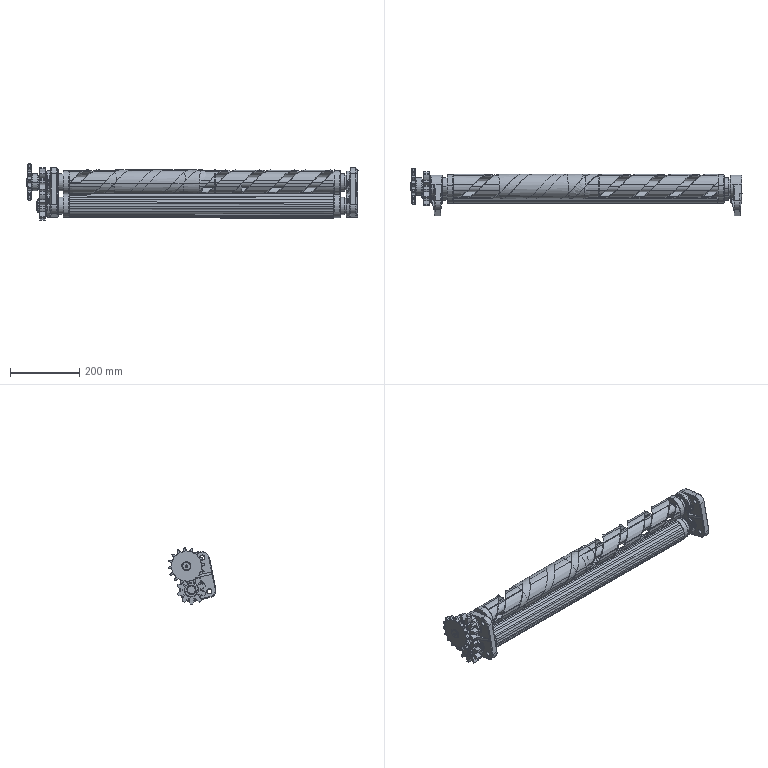Part | SolidWorks | features LayoutProfileFeature 1 | 26 solids | 1428 faces | box 961.837 x 138.935 x 163.978 mm | volume 7248262 mm3 | cylinder 656 | plane 344 | spline 293 | cone 135 | commonest cylinder face diameters 4 x74 70 x58 65 x48 76.673 x44 19.857 x34 31.085 x32